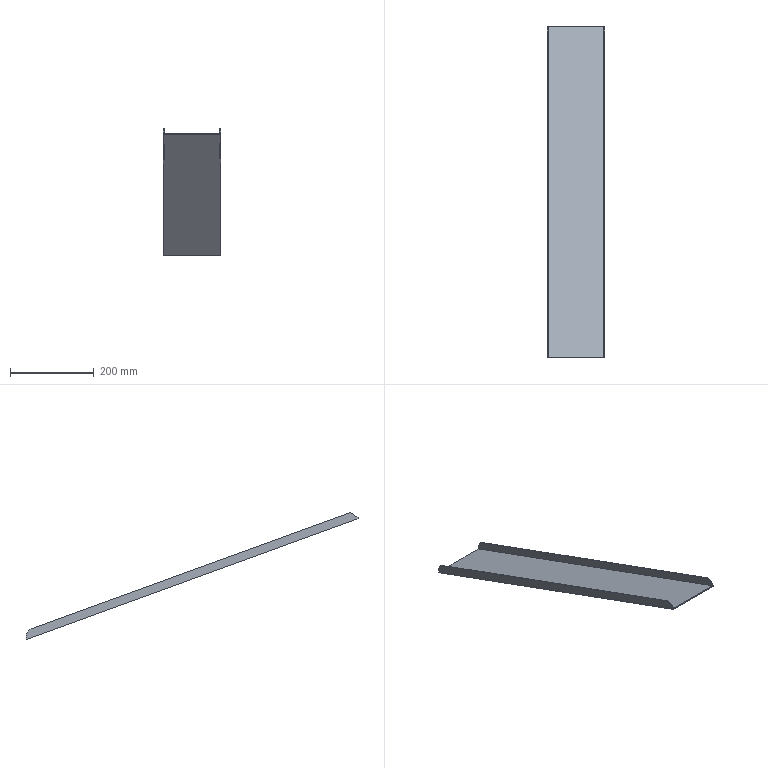Part | NX | features solid 2 | 1 solid | 14 faces | box 135.956 x 790.681 x 302.472 mm | volume 288268 mm3 | plane 12 | cylinder 2 | commonest cylinder face diameters 40 x2
STEP:
#1=CARTESIAN_POINT('',(-608.,820.,-519.765));
#2=VERTEX_POINT('',#1);
#3=CARTESIAN_POINT('',(-476.044,820.,-519.765));
#4=VERTEX_POINT('',#3);
#5=CARTESIAN_POINT('',(-698.088,820.,-519.765));
#6=DIRECTION('',(-1.,0.,0.));
#7=VECTOR('',#6,1000.);
#8=LINE('',#5,#7);
#9=EDGE_CURVE('',#2,#4,#8,.F.);
#10=ORIENTED_EDGE('',*,*,#9,.F.);
#11=CARTESIAN_POINT('',(-608.,820.,-517.637));
#12=VERTEX_POINT('',#11);
#13=CARTESIAN_POINT('',(-608.,820.,-708.));
#14=DIRECTION('',(0.,0.,-1.));
#15=VECTOR('',#14,1000.);
#16=LINE('',#13,#15);
#17=EDGE_CURVE('',#2,#12,#16,.F.);
#18=ORIENTED_EDGE('',*,*,#17,.T.);
#19=CARTESIAN_POINT('',(-476.044,820.,-517.637));
#20=VERTEX_POINT('',#19);
#21=CARTESIAN_POINT('',(370.956,820.,-517.637));
#22=DIRECTION('',(1.,0.,0.));
#23=VECTOR('',#22,1000.);
#24=LINE('',#21,#23);
#25=EDGE_CURVE('',#20,#12,#24,.F.);
#26=ORIENTED_EDGE('',*,*,#25,.F.);
#27=CARTESIAN_POINT('',(-476.044,820.,-708.));
#28=DIRECTION('',(0.,0.,-1.));
#29=VECTOR('',#28,1000.);
#30=LINE('',#27,#29);
#31=EDGE_CURVE('',#4,#20,#30,.F.);
#32=ORIENTED_EDGE('',*,*,#31,.F.);
#33=EDGE_LOOP('',(#10,#18,#26,#32));
#34=FACE_BOUND('',#33,.T.);
#35=CARTESIAN_POINT('',(370.956,820.,-708.));
#36=DIRECTION('',(0.,-1.,0.));
#37=DIRECTION('',(-1.,0.,0.));
#38=AXIS2_PLACEMENT_3D('',#35,#36,#37);
#39=PLANE('',#38);
#40=ADVANCED_FACE('',(#34),#39,.F.);
#41=CARTESIAN_POINT('',(-608.,30.526,-230.292));
#42=VERTEX_POINT('',#41);
#43=CARTESIAN_POINT('',(-608.,1206.032,-658.141));
#44=DIRECTION('',(0.,0.9397,-0.342));
#45=VECTOR('',#44,1000.);
#46=LINE('',#43,#45);
#47=EDGE_CURVE('',#42,#12,#46,.T.);
#48=ORIENTED_EDGE('',*,*,#47,.F.);
#49=CARTESIAN_POINT('',(-476.044,30.551,-230.301));
#50=VERTEX_POINT('',#49);
#51=CARTESIAN_POINT('',(-697.837,30.509,-230.285));
#52=DIRECTION('',(-1.,-0.000189,0.00006878));
#53=VECTOR('',#52,1000.);
#54=LINE('',#51,#53);
#55=EDGE_CURVE('',#42,#50,#54,.F.);
#56=ORIENTED_EDGE('',*,*,#55,.T.);
#57=CARTESIAN_POINT('',(-476.044,1206.032,-658.141));
#58=DIRECTION('',(0.,0.9397,-0.342));
#59=VECTOR('',#58,1000.);
#60=LINE('',#57,#59);
#61=EDGE_CURVE('',#50,#20,#60,.T.);
#62=ORIENTED_EDGE('',*,*,#61,.T.);
#63=ORIENTED_EDGE('',*,*,#25,.T.);
#64=EDGE_LOOP('',(#48,#56,#62,#63));
#65=FACE_BOUND('',#64,.T.);
#66=CARTESIAN_POINT('',(-698.088,1206.032,-658.141));
#67=DIRECTION('',(0.,-0.342,-0.9397));
#68=DIRECTION('',(-1.,0.,0.));
#69=AXIS2_PLACEMENT_3D('',#66,#67,#68);
#70=PLANE('',#69);
#71=ADVANCED_FACE('',(#65),#70,.F.);
#72=CARTESIAN_POINT('',(-474.044,808.047,-494.131));
#73=VERTEX_POINT('',#72);
#74=CARTESIAN_POINT('',(-474.044,47.466,-217.302));
#75=VERTEX_POINT('',#74);
#76=CARTESIAN_POINT('',(-474.044,826.84,-500.971));
#77=DIRECTION('',(0.,-0.9397,0.342));
#78=VECTOR('',#77,1000.);
#79=LINE('',#76,#78);
#80=EDGE_CURVE('',#73,#75,#79,.T.);
#81=ORIENTED_EDGE('',*,*,#80,.T.);
#82=CARTESIAN_POINT('',(-474.044,30.551,-229.146));
#83=VERTEX_POINT('',#82);
#84=CARTESIAN_POINT('',(-474.044,617.749,182.015));
#85=DIRECTION('',(0.,-0.8192,-0.5736));
#86=VECTOR('',#85,1000.);
#87=LINE('',#84,#86);
#88=EDGE_CURVE('',#75,#83,#87,.T.);
#89=ORIENTED_EDGE('',*,*,#88,.T.);
#90=CARTESIAN_POINT('',(-474.044,30.551,-232.429));
#91=VERTEX_POINT('',#90);
#92=CARTESIAN_POINT('',(-474.044,30.551,-658.141));
#93=DIRECTION('',(0.,0.,-1.));
#94=VECTOR('',#93,1000.);
#95=LINE('',#92,#94);
#96=EDGE_CURVE('',#91,#83,#95,.F.);
#97=ORIENTED_EDGE('',*,*,#96,.F.);
#98=CARTESIAN_POINT('',(-474.044,820.,-519.765));
#99=VERTEX_POINT('',#98);
#100=CARTESIAN_POINT('',(-474.044,1205.348,-660.02));
#101=DIRECTION('',(0.,-0.9397,0.342));
#102=VECTOR('',#101,1000.);
#103=LINE('',#100,#102);
#104=EDGE_CURVE('',#99,#91,#103,.T.);
#105=ORIENTED_EDGE('',*,*,#104,.F.);
#106=CARTESIAN_POINT('',(-474.044,801.206,-512.925));
#107=DIRECTION('',(-1.,0.,0.));
#108=DIRECTION('',(0.,0.,1.));
#109=AXIS2_PLACEMENT_3D('',#106,#107,#108);
#110=CIRCLE('',#109,20.);
#111=EDGE_CURVE('',#99,#73,#110,.F.);
#112=ORIENTED_EDGE('',*,*,#111,.T.);
#113=EDGE_LOOP('',(#81,#89,#97,#105,#112));
#114=FACE_BOUND('',#113,.T.);
#115=CARTESIAN_POINT('',(-474.044,1206.032,-658.141));
#116=DIRECTION('',(1.,0.,0.));
#117=DIRECTION('',(0.,0.,-1.));
#118=AXIS2_PLACEMENT_3D('',#115,#116,#117);
#119=PLANE('',#118);
#120=ADVANCED_FACE('',(#114),#119,.T.);
#121=CARTESIAN_POINT('',(-610.,30.526,-232.42));
#122=VERTEX_POINT('',#121);
#123=CARTESIAN_POINT('',(-610.,30.526,-229.136));
#124=VERTEX_POINT('',#123);
#125=CARTESIAN_POINT('',(-610.,30.526,-8.));
#126=DIRECTION('',(0.,0.,1.));
#127=VECTOR('',#126,1000.);
#128=LINE('',#125,#127);
#129=EDGE_CURVE('',#122,#124,#128,.T.);
#130=ORIENTED_EDGE('',*,*,#129,.T.);
#131=CARTESIAN_POINT('',(-610.,47.44,-217.293));
#132=VERTEX_POINT('',#131);
#133=CARTESIAN_POINT('',(-610.,47.431,-217.299));
#134=DIRECTION('',(0.,-0.8192,-0.5736));
#135=VECTOR('',#134,1000.);
#136=LINE('',#133,#135);
#137=EDGE_CURVE('',#124,#132,#136,.F.);
#138=ORIENTED_EDGE('',*,*,#137,.T.);
#139=CARTESIAN_POINT('',(-610.,808.047,-494.131));
#140=VERTEX_POINT('',#139);
#141=CARTESIAN_POINT('',(-610.,-1282.943,266.927));
#142=DIRECTION('',(0.,-0.9397,0.342));
#143=VECTOR('',#142,1000.);
#144=LINE('',#141,#143);
#145=EDGE_CURVE('',#140,#132,#144,.T.);
#146=ORIENTED_EDGE('',*,*,#145,.F.);
#147=CARTESIAN_POINT('',(-610.,820.,-519.765));
#148=VERTEX_POINT('',#147);
#149=CARTESIAN_POINT('',(-610.,801.206,-512.925));
#150=DIRECTION('',(-1.,0.,0.));
#151=DIRECTION('',(0.,0.,1.));
#152=AXIS2_PLACEMENT_3D('',#149,#150,#151);
#153=CIRCLE('',#152,20.);
#154=EDGE_CURVE('',#140,#148,#153,.T.);
#155=ORIENTED_EDGE('',*,*,#154,.T.);
#156=CARTESIAN_POINT('',(-610.,1205.348,-660.02));
#157=DIRECTION('',(0.,0.9397,-0.342));
#158=VECTOR('',#157,1000.);
#159=LINE('',#156,#158);
#160=EDGE_CURVE('',#148,#122,#159,.F.);
#161=ORIENTED_EDGE('',*,*,#160,.T.);
#162=EDGE_LOOP('',(#130,#138,#146,#155,#161));
#163=FACE_BOUND('',#162,.T.);
#164=CARTESIAN_POINT('',(-610.,-1383.009,-8.));
#165=DIRECTION('',(-1.,0.,0.));
#166=DIRECTION('',(0.,0.,1.));
#167=AXIS2_PLACEMENT_3D('',#164,#165,#166);
#168=PLANE('',#167);
#169=ADVANCED_FACE('',(#163),#168,.T.);
#170=CARTESIAN_POINT('',(-697.837,30.509,-232.414));
#171=DIRECTION('',(-1.,-0.000189,0.00006878));
#172=VECTOR('',#171,1000.);
#173=LINE('',#170,#172);
#174=EDGE_CURVE('',#122,#91,#173,.F.);
#175=ORIENTED_EDGE('',*,*,#174,.F.);
#176=ORIENTED_EDGE('',*,*,#160,.F.);
#177=CARTESIAN_POINT('',(-698.088,820.,-519.765));
#178=DIRECTION('',(-1.,0.,0.));
#179=VECTOR('',#178,1000.);
#180=LINE('',#177,#179);
#181=EDGE_CURVE('',#148,#2,#180,.F.);
#182=ORIENTED_EDGE('',*,*,#181,.T.);
#183=ORIENTED_EDGE('',*,*,#9,.T.);
#184=CARTESIAN_POINT('',(-474.044,820.,-519.765));
#185=DIRECTION('',(1.,0.,0.));
#186=VECTOR('',#185,1000.);
#187=LINE('',#184,#186);
#188=EDGE_CURVE('',#99,#4,#187,.F.);
#189=ORIENTED_EDGE('',*,*,#188,.F.);
#190=ORIENTED_EDGE('',*,*,#104,.T.);
#191=EDGE_LOOP('',(#175,#176,#182,#183,#189,#190));
#192=FACE_BOUND('',#191,.T.);
#193=CARTESIAN_POINT('',(-698.088,1205.348,-660.02));
#194=DIRECTION('',(0.,-0.342,-0.9397));
#195=DIRECTION('',(-1.,0.,0.));
#196=AXIS2_PLACEMENT_3D('',#193,#194,#195);
#197=PLANE('',#196);
#198=ADVANCED_FACE('',(#192),#197,.T.);
#199=CARTESIAN_POINT('',(-476.044,808.047,-494.131));
#200=VERTEX_POINT('',#199);
#201=CARTESIAN_POINT('',(-476.044,47.465,-217.302));
#202=VERTEX_POINT('',#201);
#203=CARTESIAN_POINT('',(-476.044,826.84,-500.971));
#204=DIRECTION('',(0.,-0.9397,0.342));
#205=VECTOR('',#204,1000.);
#206=LINE('',#203,#205);
#207=EDGE_CURVE('',#200,#202,#206,.T.);
#208=ORIENTED_EDGE('',*,*,#207,.T.);
#209=CARTESIAN_POINT('',(-473.877,47.466,-217.302));
#210=DIRECTION('',(1.,0.000189,-0.00006878));
#211=VECTOR('',#210,1000.);
#212=LINE('',#209,#211);
#213=EDGE_CURVE('',#202,#75,#212,.T.);
#214=ORIENTED_EDGE('',*,*,#213,.T.);
#215=ORIENTED_EDGE('',*,*,#80,.F.);
#216=CARTESIAN_POINT('',(-474.044,808.047,-494.131));
#217=DIRECTION('',(-1.,0.,0.));
#218=VECTOR('',#217,1000.);
#219=LINE('',#216,#218);
#220=EDGE_CURVE('',#73,#200,#219,.T.);
#221=ORIENTED_EDGE('',*,*,#220,.T.);
#222=EDGE_LOOP('',(#208,#214,#215,#221));
#223=FACE_BOUND('',#222,.T.);
#224=CARTESIAN_POINT('',(-474.044,826.84,-500.971));
#225=DIRECTION('',(0.,-0.342,-0.9397));
#226=DIRECTION('',(0.,-0.9397,0.342));
#227=AXIS2_PLACEMENT_3D('',#224,#225,#226);
#228=PLANE('',#227);
#229=ADVANCED_FACE('',(#223),#228,.F.);
#230=CARTESIAN_POINT('',(-476.044,30.551,-229.145));
#231=VERTEX_POINT('',#230);
#232=CARTESIAN_POINT('',(-476.044,30.551,-519.765));
#233=DIRECTION('',(0.,0.,1.));
#234=VECTOR('',#233,1000.);
#235=LINE('',#232,#234);
#236=EDGE_CURVE('',#231,#50,#235,.F.);
#237=ORIENTED_EDGE('',*,*,#236,.F.);
#238=CARTESIAN_POINT('',(-476.044,423.733,46.163));
#239=DIRECTION('',(0.,0.8192,0.5736));
#240=VECTOR('',#239,1000.);
#241=LINE('',#238,#240);
#242=EDGE_CURVE('',#231,#202,#241,.T.);
#243=ORIENTED_EDGE('',*,*,#242,.T.);
#244=ORIENTED_EDGE('',*,*,#207,.F.);
#245=CARTESIAN_POINT('',(-476.044,801.206,-512.925));
#246=DIRECTION('',(-1.,0.,0.));
#247=DIRECTION('',(0.,0.,1.));
#248=AXIS2_PLACEMENT_3D('',#245,#246,#247);
#249=CIRCLE('',#248,20.);
#250=EDGE_CURVE('',#200,#4,#249,.T.);
#251=ORIENTED_EDGE('',*,*,#250,.T.);
#252=ORIENTED_EDGE('',*,*,#31,.T.);
#253=ORIENTED_EDGE('',*,*,#61,.F.);
#254=EDGE_LOOP('',(#237,#243,#244,#251,#252,#253));
#255=FACE_BOUND('',#254,.T.);
#256=CARTESIAN_POINT('',(-476.044,820.,-519.765));
#257=DIRECTION('',(-1.,0.,0.));
#258=DIRECTION('',(0.,0.,1.));
#259=AXIS2_PLACEMENT_3D('',#256,#257,#258);
#260=PLANE('',#259);
#261=ADVANCED_FACE('',(#255),#260,.T.);
#262=ORIENTED_EDGE('',*,*,#111,.F.);
#263=ORIENTED_EDGE('',*,*,#188,.T.);
#264=ORIENTED_EDGE('',*,*,#250,.F.);
#265=ORIENTED_EDGE('',*,*,#220,.F.);
#266=EDGE_LOOP('',(#262,#263,#264,#265));
#267=FACE_BOUND('',#266,.T.);
#268=CARTESIAN_POINT('',(-474.044,801.206,-512.925));
#269=DIRECTION('',(-1.,0.,0.));
#270=DIRECTION('',(0.,0.,1.));
#271=AXIS2_PLACEMENT_3D('',#268,#269,#270);
#272=CYLINDRICAL_SURFACE('',#271,20.);
#273=ADVANCED_FACE('',(#267),#272,.T.);
#274=ORIENTED_EDGE('',*,*,#145,.T.);
#275=CARTESIAN_POINT('',(-608.,47.44,-217.293));
#276=VERTEX_POINT('',#275);
#277=CARTESIAN_POINT('',(-608.004,47.44,-217.293));
#278=DIRECTION('',(-1.,-0.000189,0.00006878));
#279=VECTOR('',#278,1000.);
#280=LINE('',#277,#279);
#281=EDGE_CURVE('',#132,#276,#280,.F.);
#282=ORIENTED_EDGE('',*,*,#281,.T.);
#283=CARTESIAN_POINT('',(-608.,808.047,-494.131));
#284=VERTEX_POINT('',#283);
#285=CARTESIAN_POINT('',(-608.,826.84,-500.971));
#286=DIRECTION('',(0.,0.9397,-0.342));
#287=VECTOR('',#286,1000.);
#288=LINE('',#285,#287);
#289=EDGE_CURVE('',#284,#276,#288,.F.);
#290=ORIENTED_EDGE('',*,*,#289,.F.);
#291=CARTESIAN_POINT('',(-703.088,808.047,-494.131));
#292=DIRECTION('',(-1.,0.,0.));
#293=VECTOR('',#292,1000.);
#294=LINE('',#291,#293);
#295=EDGE_CURVE('',#284,#140,#294,.T.);
#296=ORIENTED_EDGE('',*,*,#295,.T.);
#297=EDGE_LOOP('',(#274,#282,#290,#296));
#298=FACE_BOUND('',#297,.T.);
#299=CARTESIAN_POINT('',(-703.088,826.84,-500.971));
#300=DIRECTION('',(0.,-0.342,-0.9397));
#301=DIRECTION('',(0.,-0.9397,0.342));
#302=AXIS2_PLACEMENT_3D('',#299,#300,#301);
#303=PLANE('',#302);
#304=ADVANCED_FACE('',(#298),#303,.F.);
#305=ORIENTED_EDGE('',*,*,#289,.T.);
#306=CARTESIAN_POINT('',(-608.,30.526,-229.136));
#307=VERTEX_POINT('',#306);
#308=CARTESIAN_POINT('',(-608.,47.431,-217.299));
#309=DIRECTION('',(0.,-0.8192,-0.5736));
#310=VECTOR('',#309,1000.);
#311=LINE('',#308,#310);
#312=EDGE_CURVE('',#276,#307,#311,.T.);
#313=ORIENTED_EDGE('',*,*,#312,.T.);
#314=CARTESIAN_POINT('',(-608.,30.526,-8.));
#315=DIRECTION('',(0.,0.,1.));
#316=VECTOR('',#315,1000.);
#317=LINE('',#314,#316);
#318=EDGE_CURVE('',#307,#42,#317,.F.);
#319=ORIENTED_EDGE('',*,*,#318,.T.);
#320=ORIENTED_EDGE('',*,*,#47,.T.);
#321=ORIENTED_EDGE('',*,*,#17,.F.);
#322=CARTESIAN_POINT('',(-608.,801.206,-512.925));
#323=DIRECTION('',(-1.,0.,0.));
#324=DIRECTION('',(0.,0.,1.));
#325=AXIS2_PLACEMENT_3D('',#322,#323,#324);
#326=CIRCLE('',#325,20.);
#327=EDGE_CURVE('',#2,#284,#326,.F.);
#328=ORIENTED_EDGE('',*,*,#327,.T.);
#329=EDGE_LOOP('',(#305,#313,#319,#320,#321,#328));
#330=FACE_BOUND('',#329,.T.);
#331=CARTESIAN_POINT('',(-608.,-1383.009,-8.));
#332=DIRECTION('',(-1.,0.,0.));
#333=DIRECTION('',(0.,0.,1.));
#334=AXIS2_PLACEMENT_3D('',#331,#332,#333);
#335=PLANE('',#334);
#336=ADVANCED_FACE('',(#330),#335,.F.);
#337=ORIENTED_EDGE('',*,*,#154,.F.);
#338=ORIENTED_EDGE('',*,*,#295,.F.);
#339=ORIENTED_EDGE('',*,*,#327,.F.);
#340=ORIENTED_EDGE('',*,*,#181,.F.);
#341=EDGE_LOOP('',(#337,#338,#339,#340));
#342=FACE_BOUND('',#341,.T.);
#343=CARTESIAN_POINT('',(-703.088,801.206,-512.925));
#344=DIRECTION('',(1.,0.,0.));
#345=DIRECTION('',(0.,0.,-1.));
#346=AXIS2_PLACEMENT_3D('',#343,#344,#345);
#347=CYLINDRICAL_SURFACE('',#346,20.);
#348=ADVANCED_FACE('',(#342),#347,.T.);
#349=ORIENTED_EDGE('',*,*,#96,.T.);
#350=CARTESIAN_POINT('',(72.201,30.654,-229.183));
#351=DIRECTION('',(1.,0.000189,-0.00006878));
#352=VECTOR('',#351,1000.);
#353=LINE('',#350,#352);
#354=EDGE_CURVE('',#83,#231,#353,.F.);
#355=ORIENTED_EDGE('',*,*,#354,.T.);
#356=ORIENTED_EDGE('',*,*,#236,.T.);
#357=ORIENTED_EDGE('',*,*,#55,.F.);
#358=ORIENTED_EDGE('',*,*,#318,.F.);
#359=CARTESIAN_POINT('',(-610.001,30.526,-229.136));
#360=DIRECTION('',(1.,0.000189,-0.00006878));
#361=VECTOR('',#360,1000.);
#362=LINE('',#359,#361);
#363=EDGE_CURVE('',#307,#124,#362,.F.);
#364=ORIENTED_EDGE('',*,*,#363,.T.);
#365=ORIENTED_EDGE('',*,*,#129,.F.);
#366=ORIENTED_EDGE('',*,*,#174,.T.);
#367=EDGE_LOOP('',(#349,#355,#356,#357,#358,#364,#365,#366));
#368=FACE_BOUND('',#367,.T.);
#369=CARTESIAN_POINT('',(72.169,30.654,-700.));
#370=DIRECTION('',(0.000189,-1.,0.));
#371=DIRECTION('',(1.,0.000189,0.));
#372=AXIS2_PLACEMENT_3D('',#369,#370,#371);
#373=PLANE('',#372);
#374=ADVANCED_FACE('',(#368),#373,.T.);
#375=ORIENTED_EDGE('',*,*,#137,.F.);
#376=ORIENTED_EDGE('',*,*,#363,.F.);
#377=ORIENTED_EDGE('',*,*,#312,.F.);
#378=ORIENTED_EDGE('',*,*,#281,.F.);
#379=EDGE_LOOP('',(#375,#376,#377,#378));
#380=FACE_BOUND('',#379,.T.);
#381=CARTESIAN_POINT('',(-702.922,47.422,-217.286));
#382=DIRECTION('',(0.0001647,-0.5736,0.8192));
#383=DIRECTION('',(0.,-0.8192,-0.5736));
#384=AXIS2_PLACEMENT_3D('',#381,#382,#383);
#385=PLANE('',#384);
#386=ADVANCED_FACE('',(#380),#385,.T.);
#387=ORIENTED_EDGE('',*,*,#242,.F.);
#388=ORIENTED_EDGE('',*,*,#354,.F.);
#389=ORIENTED_EDGE('',*,*,#88,.F.);
#390=ORIENTED_EDGE('',*,*,#213,.F.);
#391=EDGE_LOOP('',(#387,#388,#389,#390));
#392=FACE_BOUND('',#391,.T.);
#393=CARTESIAN_POINT('',(-473.877,47.466,-217.302));
#394=DIRECTION('',(0.0001647,-0.5736,0.8192));
#395=DIRECTION('',(0.,-0.8192,-0.5736));
#396=AXIS2_PLACEMENT_3D('',#393,#394,#395);
#397=PLANE('',#396);
#398=ADVANCED_FACE('',(#392),#397,.T.);
#399=CLOSED_SHELL('',(#40,#71,#120,#169,#198,#229,#261,#273,#304,#336,#348,#374,#386,#398));
#400=MANIFOLD_SOLID_BREP('',#399);
#401=(LENGTH_UNIT()NAMED_UNIT(*)SI_UNIT(.MILLI.,.METRE.));
#402=UNCERTAINTY_MEASURE_WITH_UNIT(LENGTH_MEASURE(0.00001),#401,'','');
#403=(NAMED_UNIT(*)PLANE_ANGLE_UNIT()SI_UNIT($,.RADIAN.));
#404=(NAMED_UNIT(*)SI_UNIT($,.STERADIAN.)SOLID_ANGLE_UNIT());
#405=(GEOMETRIC_REPRESENTATION_CONTEXT(3)GLOBAL_UNCERTAINTY_ASSIGNED_CONTEXT((#402))GLOBAL_UNIT_ASSIGNED_CONTEXT((#401,#403,#404))REPRESENTATION_CONTEXT('',''));
#406=ADVANCED_BREP_SHAPE_REPRESENTATION('',(#400),#405);